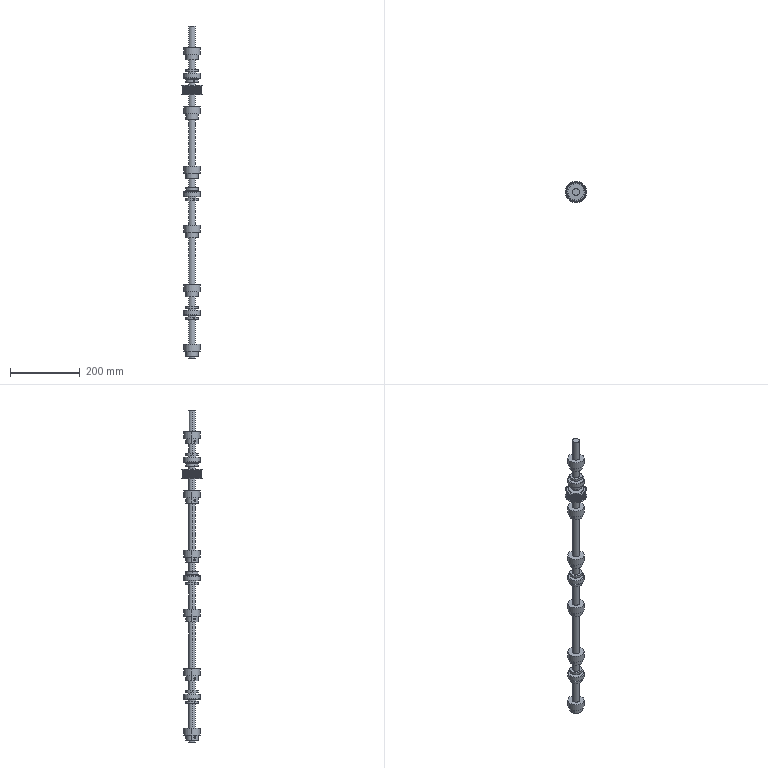Part | SolidWorks | 19 solids | 650 faces | box 61 x 61 x 952 mm | volume 663625 mm3 | cylinder 404 | plane 196 | cone 38 | torus 12 | commonest cylinder face diameters 0.8 x91 1.2 x90 52.85 x39 56.45 x36 20 x34 4.2 x24